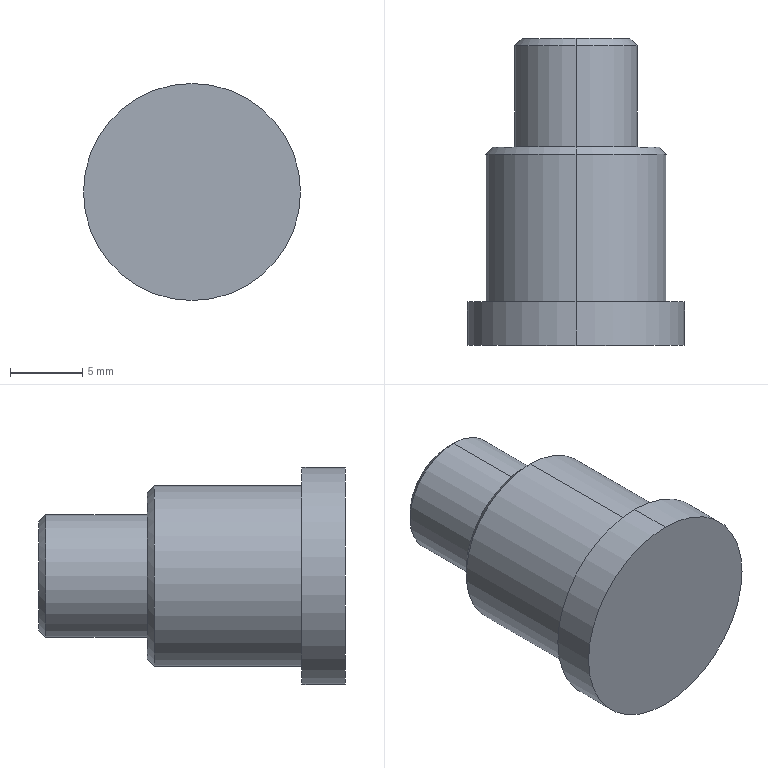Part | SolidWorks | features Chamfer 1, Revolution 1 | 1 solid | 14 faces | box 15 x 21.2 x 15 mm | volume 2261 mm3 | cylinder 6 | cone 4 | plane 4 | commonest cylinder face diameters 8.5 x2 12.5 x2 15 x2
STEP:
#1=CARTESIAN_POINT('',(-92.817,8.038,3.75));
#2=VERTEX_POINT('',#1);
#3=CARTESIAN_POINT('',(-92.817,8.038,-3.75));
#4=VERTEX_POINT('',#3);
#5=CARTESIAN_POINT('',(-92.817,8.038,0.));
#6=DIRECTION('',(0.,1.,0.));
#7=DIRECTION('',(0.,0.,1.));
#8=AXIS2_PLACEMENT_3D('',#5,#6,#7);
#9=CIRCLE('',#8,3.75);
#10=EDGE_CURVE('',#2,#4,#9,.T.);
#11=ORIENTED_EDGE('',*,*,#10,.F.);
#12=CARTESIAN_POINT('',(-92.817,7.538,4.25));
#13=VERTEX_POINT('',#12);
#14=CARTESIAN_POINT('',(-92.817,8.038,3.75));
#15=DIRECTION('',(0.,-0.7071,0.7071));
#16=VECTOR('',#15,1000.);
#17=LINE('',#14,#16);
#18=EDGE_CURVE('',#2,#13,#17,.T.);
#19=ORIENTED_EDGE('',*,*,#18,.T.);
#20=CARTESIAN_POINT('',(-92.817,7.538,-4.25));
#21=VERTEX_POINT('',#20);
#22=CARTESIAN_POINT('',(-92.817,7.538,0.));
#23=DIRECTION('',(0.,-1.,0.));
#24=DIRECTION('',(0.,0.,1.));
#25=AXIS2_PLACEMENT_3D('',#22,#23,#24);
#26=CIRCLE('',#25,4.25);
#27=EDGE_CURVE('',#21,#13,#26,.T.);
#28=ORIENTED_EDGE('',*,*,#27,.F.);
#29=CARTESIAN_POINT('',(-92.817,8.038,-3.75));
#30=DIRECTION('',(0.,-0.7071,-0.7071));
#31=VECTOR('',#30,1000.);
#32=LINE('',#29,#31);
#33=EDGE_CURVE('',#4,#21,#32,.T.);
#34=ORIENTED_EDGE('',*,*,#33,.F.);
#35=EDGE_LOOP('',(#11,#19,#28,#34));
#36=FACE_OUTER_BOUND('',#35,.T.);
#37=CARTESIAN_POINT('',(-92.817,8.038,0.));
#38=DIRECTION('',(0.,-1.,0.));
#39=DIRECTION('',(0.,0.,-1.));
#40=AXIS2_PLACEMENT_3D('',#37,#38,#39);
#41=CONICAL_SURFACE('',#40,3.75,0.7854);
#42=ADVANCED_FACE('',(#36),#41,.T.);
#43=CARTESIAN_POINT('',(-92.817,0.5382,5.75));
#44=VERTEX_POINT('',#43);
#45=CARTESIAN_POINT('',(-92.817,0.5382,-5.75));
#46=VERTEX_POINT('',#45);
#47=CARTESIAN_POINT('',(-92.817,0.5382,0.));
#48=DIRECTION('',(0.,1.,0.));
#49=DIRECTION('',(0.,0.,1.));
#50=AXIS2_PLACEMENT_3D('',#47,#48,#49);
#51=CIRCLE('',#50,5.75);
#52=EDGE_CURVE('',#44,#46,#51,.T.);
#53=ORIENTED_EDGE('',*,*,#52,.F.);
#54=CARTESIAN_POINT('',(-92.817,0.03822,6.25));
#55=VERTEX_POINT('',#54);
#56=CARTESIAN_POINT('',(-92.817,0.5382,5.75));
#57=DIRECTION('',(0.,-0.7071,0.7071));
#58=VECTOR('',#57,1000.);
#59=LINE('',#56,#58);
#60=EDGE_CURVE('',#44,#55,#59,.T.);
#61=ORIENTED_EDGE('',*,*,#60,.T.);
#62=CARTESIAN_POINT('',(-92.817,0.03822,-6.25));
#63=VERTEX_POINT('',#62);
#64=CARTESIAN_POINT('',(-92.817,0.03822,0.));
#65=DIRECTION('',(0.,-1.,0.));
#66=DIRECTION('',(0.,0.,1.));
#67=AXIS2_PLACEMENT_3D('',#64,#65,#66);
#68=CIRCLE('',#67,6.25);
#69=EDGE_CURVE('',#63,#55,#68,.T.);
#70=ORIENTED_EDGE('',*,*,#69,.F.);
#71=CARTESIAN_POINT('',(-92.817,0.5382,-5.75));
#72=DIRECTION('',(0.,-0.7071,-0.7071));
#73=VECTOR('',#72,1000.);
#74=LINE('',#71,#73);
#75=EDGE_CURVE('',#46,#63,#74,.T.);
#76=ORIENTED_EDGE('',*,*,#75,.F.);
#77=EDGE_LOOP('',(#53,#61,#70,#76));
#78=FACE_OUTER_BOUND('',#77,.T.);
#79=CARTESIAN_POINT('',(-92.817,0.5382,0.));
#80=DIRECTION('',(0.,-1.,0.));
#81=DIRECTION('',(0.,0.,-1.));
#82=AXIS2_PLACEMENT_3D('',#79,#80,#81);
#83=CONICAL_SURFACE('',#82,5.75,0.7854);
#84=ADVANCED_FACE('',(#78),#83,.T.);
#85=CARTESIAN_POINT('',(-92.817,-13.162,7.5));
#86=VERTEX_POINT('',#85);
#87=CARTESIAN_POINT('',(-92.817,-13.162,-7.5));
#88=VERTEX_POINT('',#87);
#89=CARTESIAN_POINT('',(-92.817,-13.162,0.));
#90=DIRECTION('',(0.,1.,0.));
#91=DIRECTION('',(0.,0.,1.));
#92=AXIS2_PLACEMENT_3D('',#89,#90,#91);
#93=CIRCLE('',#92,7.5);
#94=EDGE_CURVE('',#86,#88,#93,.T.);
#95=ORIENTED_EDGE('',*,*,#94,.T.);
#96=CARTESIAN_POINT('',(-92.817,-10.162,-7.5));
#97=VERTEX_POINT('',#96);
#98=CARTESIAN_POINT('',(-92.817,8.103,-7.5));
#99=DIRECTION('',(0.,1.,0.));
#100=VECTOR('',#99,1000.);
#101=LINE('',#98,#100);
#102=EDGE_CURVE('',#88,#97,#101,.T.);
#103=ORIENTED_EDGE('',*,*,#102,.T.);
#104=CARTESIAN_POINT('',(-92.817,-10.162,7.5));
#105=VERTEX_POINT('',#104);
#106=CARTESIAN_POINT('',(-92.817,-10.162,0.));
#107=DIRECTION('',(0.,1.,0.));
#108=DIRECTION('',(0.,0.,1.));
#109=AXIS2_PLACEMENT_3D('',#106,#107,#108);
#110=CIRCLE('',#109,7.5);
#111=EDGE_CURVE('',#105,#97,#110,.T.);
#112=ORIENTED_EDGE('',*,*,#111,.F.);
#113=CARTESIAN_POINT('',(-92.817,8.103,7.5));
#114=DIRECTION('',(0.,1.,0.));
#115=VECTOR('',#114,1000.);
#116=LINE('',#113,#115);
#117=EDGE_CURVE('',#86,#105,#116,.T.);
#118=ORIENTED_EDGE('',*,*,#117,.F.);
#119=EDGE_LOOP('',(#95,#103,#112,#118));
#120=FACE_OUTER_BOUND('',#119,.T.);
#121=CARTESIAN_POINT('',(-92.817,8.103,0.));
#122=DIRECTION('',(0.,1.,0.));
#123=DIRECTION('',(0.,0.,1.));
#124=AXIS2_PLACEMENT_3D('',#121,#122,#123);
#125=CYLINDRICAL_SURFACE('',#124,7.5);
#126=ADVANCED_FACE('',(#120),#125,.T.);
#127=CARTESIAN_POINT('',(-92.817,0.5382,4.25));
#128=VERTEX_POINT('',#127);
#129=CARTESIAN_POINT('',(-92.817,0.5382,-4.25));
#130=VERTEX_POINT('',#129);
#131=CARTESIAN_POINT('',(-92.817,0.5382,0.));
#132=DIRECTION('',(0.,1.,0.));
#133=DIRECTION('',(0.,0.,1.));
#134=AXIS2_PLACEMENT_3D('',#131,#132,#133);
#135=CIRCLE('',#134,4.25);
#136=EDGE_CURVE('',#128,#130,#135,.T.);
#137=ORIENTED_EDGE('',*,*,#136,.T.);
#138=CARTESIAN_POINT('',(-92.817,8.103,-4.25));
#139=DIRECTION('',(0.,1.,0.));
#140=VECTOR('',#139,1000.);
#141=LINE('',#138,#140);
#142=EDGE_CURVE('',#130,#21,#141,.T.);
#143=ORIENTED_EDGE('',*,*,#142,.T.);
#144=ORIENTED_EDGE('',*,*,#27,.T.);
#145=CARTESIAN_POINT('',(-92.817,8.103,4.25));
#146=DIRECTION('',(0.,1.,0.));
#147=VECTOR('',#146,1000.);
#148=LINE('',#145,#147);
#149=EDGE_CURVE('',#128,#13,#148,.T.);
#150=ORIENTED_EDGE('',*,*,#149,.F.);
#151=EDGE_LOOP('',(#137,#143,#144,#150));
#152=FACE_OUTER_BOUND('',#151,.T.);
#153=CARTESIAN_POINT('',(-92.817,8.103,0.));
#154=DIRECTION('',(0.,1.,0.));
#155=DIRECTION('',(0.,0.,1.));
#156=AXIS2_PLACEMENT_3D('',#153,#154,#155);
#157=CYLINDRICAL_SURFACE('',#156,4.25);
#158=ADVANCED_FACE('',(#152),#157,.T.);
#159=CARTESIAN_POINT('',(-92.817,-10.162,6.25));
#160=VERTEX_POINT('',#159);
#161=CARTESIAN_POINT('',(-92.817,-10.162,-6.25));
#162=VERTEX_POINT('',#161);
#163=CARTESIAN_POINT('',(-92.817,-10.162,0.));
#164=DIRECTION('',(0.,1.,0.));
#165=DIRECTION('',(0.,0.,1.));
#166=AXIS2_PLACEMENT_3D('',#163,#164,#165);
#167=CIRCLE('',#166,6.25);
#168=EDGE_CURVE('',#160,#162,#167,.T.);
#169=ORIENTED_EDGE('',*,*,#168,.T.);
#170=CARTESIAN_POINT('',(-92.817,8.103,-6.25));
#171=DIRECTION('',(0.,1.,0.));
#172=VECTOR('',#171,1000.);
#173=LINE('',#170,#172);
#174=EDGE_CURVE('',#162,#63,#173,.T.);
#175=ORIENTED_EDGE('',*,*,#174,.T.);
#176=ORIENTED_EDGE('',*,*,#69,.T.);
#177=CARTESIAN_POINT('',(-92.817,8.103,6.25));
#178=DIRECTION('',(0.,1.,0.));
#179=VECTOR('',#178,1000.);
#180=LINE('',#177,#179);
#181=EDGE_CURVE('',#160,#55,#180,.T.);
#182=ORIENTED_EDGE('',*,*,#181,.F.);
#183=EDGE_LOOP('',(#169,#175,#176,#182));
#184=FACE_OUTER_BOUND('',#183,.T.);
#185=CARTESIAN_POINT('',(-92.817,8.103,0.));
#186=DIRECTION('',(0.,1.,0.));
#187=DIRECTION('',(0.,0.,1.));
#188=AXIS2_PLACEMENT_3D('',#185,#186,#187);
#189=CYLINDRICAL_SURFACE('',#188,6.25);
#190=ADVANCED_FACE('',(#184),#189,.T.);
#191=ORIENTED_EDGE('',*,*,#174,.F.);
#192=CARTESIAN_POINT('',(-92.817,-10.162,0.));
#193=DIRECTION('',(0.,1.,0.));
#194=DIRECTION('',(0.,0.,1.));
#195=AXIS2_PLACEMENT_3D('',#192,#193,#194);
#196=CIRCLE('',#195,6.25);
#197=EDGE_CURVE('',#162,#160,#196,.T.);
#198=ORIENTED_EDGE('',*,*,#197,.T.);
#199=ORIENTED_EDGE('',*,*,#181,.T.);
#200=CARTESIAN_POINT('',(-92.817,0.03822,0.));
#201=DIRECTION('',(0.,-1.,0.));
#202=DIRECTION('',(0.,0.,1.));
#203=AXIS2_PLACEMENT_3D('',#200,#201,#202);
#204=CIRCLE('',#203,6.25);
#205=EDGE_CURVE('',#55,#63,#204,.T.);
#206=ORIENTED_EDGE('',*,*,#205,.T.);
#207=EDGE_LOOP('',(#191,#198,#199,#206));
#208=FACE_OUTER_BOUND('',#207,.T.);
#209=CARTESIAN_POINT('',(-92.817,8.103,0.));
#210=DIRECTION('',(0.,1.,0.));
#211=DIRECTION('',(0.,0.,1.));
#212=AXIS2_PLACEMENT_3D('',#209,#210,#211);
#213=CYLINDRICAL_SURFACE('',#212,6.25);
#214=ADVANCED_FACE('',(#208),#213,.T.);
#215=CARTESIAN_POINT('',(-92.817,0.5382,0.));
#216=DIRECTION('',(0.,1.,0.));
#217=DIRECTION('',(0.,0.,1.));
#218=AXIS2_PLACEMENT_3D('',#215,#216,#217);
#219=CIRCLE('',#218,5.75);
#220=EDGE_CURVE('',#46,#44,#219,.T.);
#221=ORIENTED_EDGE('',*,*,#220,.T.);
#222=ORIENTED_EDGE('',*,*,#52,.T.);
#223=EDGE_LOOP('',(#221,#222));
#224=FACE_OUTER_BOUND('',#223,.T.);
#225=ORIENTED_EDGE('',*,*,#136,.F.);
#226=CARTESIAN_POINT('',(-92.817,0.5382,0.));
#227=DIRECTION('',(0.,1.,0.));
#228=DIRECTION('',(0.,0.,1.));
#229=AXIS2_PLACEMENT_3D('',#226,#227,#228);
#230=CIRCLE('',#229,4.25);
#231=EDGE_CURVE('',#130,#128,#230,.T.);
#232=ORIENTED_EDGE('',*,*,#231,.F.);
#233=EDGE_LOOP('',(#225,#232));
#234=FACE_BOUND('',#233,.T.);
#235=CARTESIAN_POINT('',(-99.067,0.5382,0.));
#236=DIRECTION('',(0.,1.,0.));
#237=DIRECTION('',(0.,0.,1.));
#238=AXIS2_PLACEMENT_3D('',#235,#236,#237);
#239=PLANE('',#238);
#240=ADVANCED_FACE('',(#224,#234),#239,.T.);
#241=ORIENTED_EDGE('',*,*,#142,.F.);
#242=ORIENTED_EDGE('',*,*,#231,.T.);
#243=ORIENTED_EDGE('',*,*,#149,.T.);
#244=CARTESIAN_POINT('',(-92.817,7.538,0.));
#245=DIRECTION('',(0.,-1.,0.));
#246=DIRECTION('',(0.,0.,1.));
#247=AXIS2_PLACEMENT_3D('',#244,#245,#246);
#248=CIRCLE('',#247,4.25);
#249=EDGE_CURVE('',#13,#21,#248,.T.);
#250=ORIENTED_EDGE('',*,*,#249,.T.);
#251=EDGE_LOOP('',(#241,#242,#243,#250));
#252=FACE_OUTER_BOUND('',#251,.T.);
#253=CARTESIAN_POINT('',(-92.817,8.103,0.));
#254=DIRECTION('',(0.,1.,0.));
#255=DIRECTION('',(0.,0.,1.));
#256=AXIS2_PLACEMENT_3D('',#253,#254,#255);
#257=CYLINDRICAL_SURFACE('',#256,4.25);
#258=ADVANCED_FACE('',(#252),#257,.T.);
#259=CARTESIAN_POINT('',(-92.817,8.038,0.));
#260=DIRECTION('',(0.,1.,0.));
#261=DIRECTION('',(0.,0.,1.));
#262=AXIS2_PLACEMENT_3D('',#259,#260,#261);
#263=CIRCLE('',#262,3.75);
#264=EDGE_CURVE('',#4,#2,#263,.T.);
#265=ORIENTED_EDGE('',*,*,#264,.T.);
#266=ORIENTED_EDGE('',*,*,#10,.T.);
#267=EDGE_LOOP('',(#265,#266));
#268=FACE_OUTER_BOUND('',#267,.T.);
#269=CARTESIAN_POINT('',(-97.067,8.038,0.));
#270=DIRECTION('',(0.,1.,0.));
#271=DIRECTION('',(0.,0.,1.));
#272=AXIS2_PLACEMENT_3D('',#269,#270,#271);
#273=PLANE('',#272);
#274=ADVANCED_FACE('',(#268),#273,.T.);
#275=ORIENTED_EDGE('',*,*,#94,.F.);
#276=CARTESIAN_POINT('',(-92.817,-13.162,0.));
#277=DIRECTION('',(0.,1.,0.));
#278=DIRECTION('',(0.,0.,1.));
#279=AXIS2_PLACEMENT_3D('',#276,#277,#278);
#280=CIRCLE('',#279,7.5);
#281=EDGE_CURVE('',#88,#86,#280,.T.);
#282=ORIENTED_EDGE('',*,*,#281,.F.);
#283=EDGE_LOOP('',(#275,#282));
#284=FACE_OUTER_BOUND('',#283,.T.);
#285=CARTESIAN_POINT('',(-100.317,-13.162,0.));
#286=DIRECTION('',(0.,-1.,0.));
#287=DIRECTION('',(0.,0.,-1.));
#288=AXIS2_PLACEMENT_3D('',#285,#286,#287);
#289=PLANE('',#288);
#290=ADVANCED_FACE('',(#284),#289,.T.);
#291=ORIENTED_EDGE('',*,*,#102,.F.);
#292=ORIENTED_EDGE('',*,*,#281,.T.);
#293=ORIENTED_EDGE('',*,*,#117,.T.);
#294=CARTESIAN_POINT('',(-92.817,-10.162,0.));
#295=DIRECTION('',(0.,1.,0.));
#296=DIRECTION('',(0.,0.,1.));
#297=AXIS2_PLACEMENT_3D('',#294,#295,#296);
#298=CIRCLE('',#297,7.5);
#299=EDGE_CURVE('',#97,#105,#298,.T.);
#300=ORIENTED_EDGE('',*,*,#299,.F.);
#301=EDGE_LOOP('',(#291,#292,#293,#300));
#302=FACE_OUTER_BOUND('',#301,.T.);
#303=CARTESIAN_POINT('',(-92.817,8.103,0.));
#304=DIRECTION('',(0.,1.,0.));
#305=DIRECTION('',(0.,0.,1.));
#306=AXIS2_PLACEMENT_3D('',#303,#304,#305);
#307=CYLINDRICAL_SURFACE('',#306,7.5);
#308=ADVANCED_FACE('',(#302),#307,.T.);
#309=ORIENTED_EDGE('',*,*,#111,.T.);
#310=ORIENTED_EDGE('',*,*,#299,.T.);
#311=EDGE_LOOP('',(#309,#310));
#312=FACE_OUTER_BOUND('',#311,.T.);
#313=ORIENTED_EDGE('',*,*,#168,.F.);
#314=ORIENTED_EDGE('',*,*,#197,.F.);
#315=EDGE_LOOP('',(#313,#314));
#316=FACE_BOUND('',#315,.T.);
#317=CARTESIAN_POINT('',(-99.067,-10.162,0.));
#318=DIRECTION('',(0.,1.,0.));
#319=DIRECTION('',(0.,0.,1.));
#320=AXIS2_PLACEMENT_3D('',#317,#318,#319);
#321=PLANE('',#320);
#322=ADVANCED_FACE('',(#312,#316),#321,.T.);
#323=ORIENTED_EDGE('',*,*,#60,.F.);
#324=ORIENTED_EDGE('',*,*,#220,.F.);
#325=ORIENTED_EDGE('',*,*,#75,.T.);
#326=ORIENTED_EDGE('',*,*,#205,.F.);
#327=EDGE_LOOP('',(#323,#324,#325,#326));
#328=FACE_OUTER_BOUND('',#327,.T.);
#329=CARTESIAN_POINT('',(-92.817,0.5382,0.));
#330=DIRECTION('',(0.,-1.,0.));
#331=DIRECTION('',(0.,0.,-1.));
#332=AXIS2_PLACEMENT_3D('',#329,#330,#331);
#333=CONICAL_SURFACE('',#332,5.75,0.7854);
#334=ADVANCED_FACE('',(#328),#333,.T.);
#335=ORIENTED_EDGE('',*,*,#18,.F.);
#336=ORIENTED_EDGE('',*,*,#264,.F.);
#337=ORIENTED_EDGE('',*,*,#33,.T.);
#338=ORIENTED_EDGE('',*,*,#249,.F.);
#339=EDGE_LOOP('',(#335,#336,#337,#338));
#340=FACE_OUTER_BOUND('',#339,.T.);
#341=CARTESIAN_POINT('',(-92.817,8.038,0.));
#342=DIRECTION('',(0.,-1.,0.));
#343=DIRECTION('',(0.,0.,-1.));
#344=AXIS2_PLACEMENT_3D('',#341,#342,#343);
#345=CONICAL_SURFACE('',#344,3.75,0.7854);
#346=ADVANCED_FACE('',(#340),#345,.T.);
#347=CLOSED_SHELL('',(#42,#84,#126,#158,#190,#214,#240,#258,#274,#290,#308,#322,#334,#346));
#348=MANIFOLD_SOLID_BREP('',#347);
#349=CARTESIAN_POINT('',(0.,0.,0.));
#350=DIRECTION('',(0.,0.,1.));
#351=DIRECTION('',(1.,0.,0.));
#352=AXIS2_PLACEMENT_3D('',#349,#350,#351);
#353=(LENGTH_UNIT()NAMED_UNIT(*)SI_UNIT(.MILLI.,.METRE.));
#354=UNCERTAINTY_MEASURE_WITH_UNIT(LENGTH_MEASURE(0.00001),#353,'','');
#355=(NAMED_UNIT(*)PLANE_ANGLE_UNIT()SI_UNIT($,.RADIAN.));
#356=(NAMED_UNIT(*)SI_UNIT($,.STERADIAN.)SOLID_ANGLE_UNIT());
#357=(GEOMETRIC_REPRESENTATION_CONTEXT(3)GLOBAL_UNCERTAINTY_ASSIGNED_CONTEXT((#354))GLOBAL_UNIT_ASSIGNED_CONTEXT((#353,#355,#356))REPRESENTATION_CONTEXT('',''));
#358=ADVANCED_BREP_SHAPE_REPRESENTATION('',(#348,#352),#357);